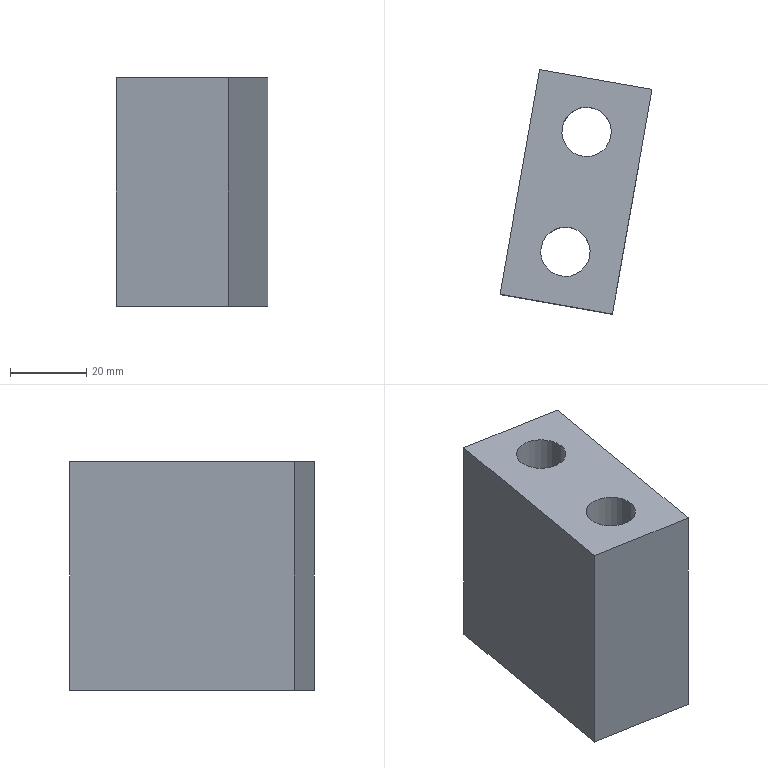Part | NX | features solid 2 | 1 solid | 12 faces | box 39.963 x 64.298 x 60 mm | volume 84815 mm3 | plane 8 | cylinder 4 | commonest cylinder face diameters 13 x2 20 x2
STEP:
#1=CARTESIAN_POINT('',(487.163,-102.147,147.5));
#2=VERTEX_POINT('',#1);
#3=CARTESIAN_POINT('',(493.565,-103.276,147.5));
#4=DIRECTION('',(0.,0.,-1.));
#5=DIRECTION('',(-0.9848,0.1736,0.));
#6=AXIS2_PLACEMENT_3D('',#3,#4,#5);
#7=CIRCLE('',#6,6.5);
#8=EDGE_CURVE('',#2,#2,#7,.F.);
#9=ORIENTED_EDGE('',*,*,#8,.F.);
#10=EDGE_LOOP('',(#9));
#11=FACE_BOUND('',#10,.T.);
#12=CARTESIAN_POINT('',(492.72,-70.633,147.5));
#13=VERTEX_POINT('',#12);
#14=CARTESIAN_POINT('',(499.121,-71.762,147.5));
#15=DIRECTION('',(0.,0.,-1.));
#16=DIRECTION('',(-0.9848,0.1736,0.));
#17=AXIS2_PLACEMENT_3D('',#14,#15,#16);
#18=CIRCLE('',#17,6.5);
#19=EDGE_CURVE('',#13,#13,#18,.F.);
#20=ORIENTED_EDGE('',*,*,#19,.F.);
#21=EDGE_LOOP('',(#20));
#22=FACE_BOUND('',#21,.T.);
#23=CARTESIAN_POINT('',(486.78,-55.37,147.5));
#24=VERTEX_POINT('',#23);
#25=CARTESIAN_POINT('',(516.325,-60.579,147.5));
#26=VERTEX_POINT('',#25);
#27=CARTESIAN_POINT('',(481.856,-54.501,147.5));
#28=DIRECTION('',(-0.9848,0.1736,0.));
#29=VECTOR('',#28,1000.);
#30=LINE('',#27,#29);
#31=EDGE_CURVE('',#24,#26,#30,.F.);
#32=ORIENTED_EDGE('',*,*,#31,.F.);
#33=CARTESIAN_POINT('',(476.362,-114.458,147.5));
#34=VERTEX_POINT('',#33);
#35=CARTESIAN_POINT('',(476.362,-114.458,147.5));
#36=DIRECTION('',(-0.1736,-0.9848,0.));
#37=VECTOR('',#36,1000.);
#38=LINE('',#35,#37);
#39=EDGE_CURVE('',#34,#24,#38,.F.);
#40=ORIENTED_EDGE('',*,*,#39,.F.);
#41=CARTESIAN_POINT('',(505.906,-119.668,147.5));
#42=VERTEX_POINT('',#41);
#43=CARTESIAN_POINT('',(471.438,-113.59,147.5));
#44=DIRECTION('',(-0.9848,0.1736,0.));
#45=VECTOR('',#44,1000.);
#46=LINE('',#43,#45);
#47=EDGE_CURVE('',#34,#42,#46,.F.);
#48=ORIENTED_EDGE('',*,*,#47,.T.);
#49=CARTESIAN_POINT('',(505.906,-119.668,147.5));
#50=DIRECTION('',(-0.1736,-0.9848,0.));
#51=VECTOR('',#50,1000.);
#52=LINE('',#49,#51);
#53=EDGE_CURVE('',#42,#26,#52,.F.);
#54=ORIENTED_EDGE('',*,*,#53,.T.);
#55=EDGE_LOOP('',(#32,#40,#48,#54));
#56=FACE_BOUND('',#55,.T.);
#57=CARTESIAN_POINT('',(471.438,-113.59,147.5));
#58=DIRECTION('',(0.,0.,1.));
#59=DIRECTION('',(0.1736,0.9848,0.));
#60=AXIS2_PLACEMENT_3D('',#57,#58,#59);
#61=PLANE('',#60);
#62=ADVANCED_FACE('',(#11,#22,#56),#61,.T.);
#63=ORIENTED_EDGE('',*,*,#47,.F.);
#64=CARTESIAN_POINT('',(476.362,-114.458,87.5));
#65=VERTEX_POINT('',#64);
#66=CARTESIAN_POINT('',(476.362,-114.458,147.5));
#67=DIRECTION('',(0.,0.,-1.));
#68=VECTOR('',#67,1000.);
#69=LINE('',#66,#68);
#70=EDGE_CURVE('',#34,#65,#69,.T.);
#71=ORIENTED_EDGE('',*,*,#70,.T.);
#72=CARTESIAN_POINT('',(505.906,-119.668,87.5));
#73=VERTEX_POINT('',#72);
#74=CARTESIAN_POINT('',(471.438,-113.59,87.5));
#75=DIRECTION('',(0.9848,-0.1736,0.));
#76=VECTOR('',#75,1000.);
#77=LINE('',#74,#76);
#78=EDGE_CURVE('',#65,#73,#77,.T.);
#79=ORIENTED_EDGE('',*,*,#78,.T.);
#80=CARTESIAN_POINT('',(505.906,-119.668,147.5));
#81=DIRECTION('',(0.,0.,-1.));
#82=VECTOR('',#81,1000.);
#83=LINE('',#80,#82);
#84=EDGE_CURVE('',#42,#73,#83,.T.);
#85=ORIENTED_EDGE('',*,*,#84,.F.);
#86=EDGE_LOOP('',(#63,#71,#79,#85));
#87=FACE_BOUND('',#86,.T.);
#88=CARTESIAN_POINT('',(471.438,-113.59,147.5));
#89=DIRECTION('',(0.1736,0.9848,0.));
#90=DIRECTION('',(0.,0.,-1.));
#91=AXIS2_PLACEMENT_3D('',#88,#89,#90);
#92=PLANE('',#91);
#93=ADVANCED_FACE('',(#87),#92,.F.);
#94=CARTESIAN_POINT('',(483.717,-101.539,87.5));
#95=VERTEX_POINT('',#94);
#96=CARTESIAN_POINT('',(493.565,-103.276,87.5));
#97=DIRECTION('',(0.,0.,-1.));
#98=DIRECTION('',(-0.9848,0.1736,0.));
#99=AXIS2_PLACEMENT_3D('',#96,#97,#98);
#100=CIRCLE('',#99,10.);
#101=EDGE_CURVE('',#95,#95,#100,.T.);
#102=ORIENTED_EDGE('',*,*,#101,.F.);
#103=EDGE_LOOP('',(#102));
#104=FACE_BOUND('',#103,.T.);
#105=CARTESIAN_POINT('',(489.273,-70.025,87.5));
#106=VERTEX_POINT('',#105);
#107=CARTESIAN_POINT('',(499.121,-71.762,87.5));
#108=DIRECTION('',(0.,0.,-1.));
#109=DIRECTION('',(-0.9848,0.1736,0.));
#110=AXIS2_PLACEMENT_3D('',#107,#108,#109);
#111=CIRCLE('',#110,10.);
#112=EDGE_CURVE('',#106,#106,#111,.T.);
#113=ORIENTED_EDGE('',*,*,#112,.F.);
#114=EDGE_LOOP('',(#113));
#115=FACE_BOUND('',#114,.T.);
#116=ORIENTED_EDGE('',*,*,#78,.F.);
#117=CARTESIAN_POINT('',(486.78,-55.37,87.5));
#118=VERTEX_POINT('',#117);
#119=CARTESIAN_POINT('',(476.362,-114.458,87.5));
#120=DIRECTION('',(0.1736,0.9848,0.));
#121=VECTOR('',#120,1000.);
#122=LINE('',#119,#121);
#123=EDGE_CURVE('',#65,#118,#122,.T.);
#124=ORIENTED_EDGE('',*,*,#123,.T.);
#125=CARTESIAN_POINT('',(516.325,-60.579,87.5));
#126=VERTEX_POINT('',#125);
#127=CARTESIAN_POINT('',(481.856,-54.501,87.5));
#128=DIRECTION('',(-0.9848,0.1736,0.));
#129=VECTOR('',#128,1000.);
#130=LINE('',#127,#129);
#131=EDGE_CURVE('',#118,#126,#130,.F.);
#132=ORIENTED_EDGE('',*,*,#131,.T.);
#133=CARTESIAN_POINT('',(505.906,-119.668,87.5));
#134=DIRECTION('',(0.1736,0.9848,0.));
#135=VECTOR('',#134,1000.);
#136=LINE('',#133,#135);
#137=EDGE_CURVE('',#73,#126,#136,.T.);
#138=ORIENTED_EDGE('',*,*,#137,.F.);
#139=EDGE_LOOP('',(#116,#124,#132,#138));
#140=FACE_BOUND('',#139,.T.);
#141=CARTESIAN_POINT('',(471.438,-113.59,87.5));
#142=DIRECTION('',(0.,0.,1.));
#143=DIRECTION('',(0.1736,0.9848,0.));
#144=AXIS2_PLACEMENT_3D('',#141,#142,#143);
#145=PLANE('',#144);
#146=ADVANCED_FACE('',(#104,#115,#140),#145,.F.);
#147=CARTESIAN_POINT('',(486.78,-55.37,147.5));
#148=DIRECTION('',(0.,0.,1.));
#149=VECTOR('',#148,1000.);
#150=LINE('',#147,#149);
#151=EDGE_CURVE('',#24,#118,#150,.F.);
#152=ORIENTED_EDGE('',*,*,#151,.F.);
#153=ORIENTED_EDGE('',*,*,#31,.T.);
#154=CARTESIAN_POINT('',(516.325,-60.579,147.5));
#155=DIRECTION('',(0.,0.,1.));
#156=VECTOR('',#155,1000.);
#157=LINE('',#154,#156);
#158=EDGE_CURVE('',#26,#126,#157,.F.);
#159=ORIENTED_EDGE('',*,*,#158,.T.);
#160=ORIENTED_EDGE('',*,*,#131,.F.);
#161=EDGE_LOOP('',(#152,#153,#159,#160));
#162=FACE_BOUND('',#161,.T.);
#163=CARTESIAN_POINT('',(481.856,-54.501,147.5));
#164=DIRECTION('',(0.1736,0.9848,0.));
#165=DIRECTION('',(0.,0.,-1.));
#166=AXIS2_PLACEMENT_3D('',#163,#164,#165);
#167=PLANE('',#166);
#168=ADVANCED_FACE('',(#162),#167,.T.);
#169=ORIENTED_EDGE('',*,*,#137,.T.);
#170=ORIENTED_EDGE('',*,*,#158,.F.);
#171=ORIENTED_EDGE('',*,*,#53,.F.);
#172=ORIENTED_EDGE('',*,*,#84,.T.);
#173=EDGE_LOOP('',(#169,#170,#171,#172));
#174=FACE_BOUND('',#173,.T.);
#175=CARTESIAN_POINT('',(505.906,-119.668,147.5));
#176=DIRECTION('',(0.9848,-0.1736,0.));
#177=DIRECTION('',(0.,0.,1.));
#178=AXIS2_PLACEMENT_3D('',#175,#176,#177);
#179=PLANE('',#178);
#180=ADVANCED_FACE('',(#174),#179,.T.);
#181=ORIENTED_EDGE('',*,*,#123,.F.);
#182=ORIENTED_EDGE('',*,*,#70,.F.);
#183=ORIENTED_EDGE('',*,*,#39,.T.);
#184=ORIENTED_EDGE('',*,*,#151,.T.);
#185=EDGE_LOOP('',(#181,#182,#183,#184));
#186=FACE_BOUND('',#185,.T.);
#187=CARTESIAN_POINT('',(476.362,-114.458,147.5));
#188=DIRECTION('',(0.9848,-0.1736,0.));
#189=DIRECTION('',(0.,0.,1.));
#190=AXIS2_PLACEMENT_3D('',#187,#188,#189);
#191=PLANE('',#190);
#192=ADVANCED_FACE('',(#186),#191,.F.);
#193=CARTESIAN_POINT('',(492.72,-70.633,107.5));
#194=VERTEX_POINT('',#193);
#195=CARTESIAN_POINT('',(499.121,-71.762,107.5));
#196=DIRECTION('',(0.,0.,-1.));
#197=DIRECTION('',(-0.9848,0.1736,0.));
#198=AXIS2_PLACEMENT_3D('',#195,#196,#197);
#199=CIRCLE('',#198,6.5);
#200=EDGE_CURVE('',#194,#194,#199,.T.);
#201=ORIENTED_EDGE('',*,*,#200,.T.);
#202=EDGE_LOOP('',(#201));
#203=FACE_BOUND('',#202,.T.);
#204=ORIENTED_EDGE('',*,*,#19,.T.);
#205=EDGE_LOOP('',(#204));
#206=FACE_BOUND('',#205,.T.);
#207=CARTESIAN_POINT('',(499.121,-71.762,167.5));
#208=DIRECTION('',(0.,0.,1.));
#209=DIRECTION('',(-0.9848,0.1736,0.));
#210=AXIS2_PLACEMENT_3D('',#207,#208,#209);
#211=CYLINDRICAL_SURFACE('',#210,6.5);
#212=ADVANCED_FACE('',(#203,#206),#211,.F.);
#213=ORIENTED_EDGE('',*,*,#200,.F.);
#214=EDGE_LOOP('',(#213));
#215=FACE_BOUND('',#214,.T.);
#216=CARTESIAN_POINT('',(489.273,-70.025,107.5));
#217=VERTEX_POINT('',#216);
#218=CARTESIAN_POINT('',(499.121,-71.762,107.5));
#219=DIRECTION('',(0.,0.,-1.));
#220=DIRECTION('',(-0.9848,0.1736,0.));
#221=AXIS2_PLACEMENT_3D('',#218,#219,#220);
#222=CIRCLE('',#221,10.);
#223=EDGE_CURVE('',#217,#217,#222,.T.);
#224=ORIENTED_EDGE('',*,*,#223,.T.);
#225=EDGE_LOOP('',(#224));
#226=FACE_BOUND('',#225,.T.);
#227=CARTESIAN_POINT('',(499.469,-69.792,107.5));
#228=DIRECTION('',(0.,0.,1.));
#229=DIRECTION('',(-0.9848,0.1736,0.));
#230=AXIS2_PLACEMENT_3D('',#227,#228,#229);
#231=PLANE('',#230);
#232=ADVANCED_FACE('',(#215,#226),#231,.F.);
#233=ORIENTED_EDGE('',*,*,#223,.F.);
#234=EDGE_LOOP('',(#233));
#235=FACE_BOUND('',#234,.T.);
#236=ORIENTED_EDGE('',*,*,#112,.T.);
#237=EDGE_LOOP('',(#236));
#238=FACE_BOUND('',#237,.T.);
#239=CARTESIAN_POINT('',(499.121,-71.762,87.5));
#240=DIRECTION('',(0.,0.,1.));
#241=DIRECTION('',(-0.9848,0.1736,0.));
#242=AXIS2_PLACEMENT_3D('',#239,#240,#241);
#243=CYLINDRICAL_SURFACE('',#242,10.);
#244=ADVANCED_FACE('',(#235,#238),#243,.F.);
#245=CARTESIAN_POINT('',(487.163,-102.147,107.5));
#246=VERTEX_POINT('',#245);
#247=CARTESIAN_POINT('',(493.565,-103.276,107.5));
#248=DIRECTION('',(0.,0.,-1.));
#249=DIRECTION('',(-0.9848,0.1736,0.));
#250=AXIS2_PLACEMENT_3D('',#247,#248,#249);
#251=CIRCLE('',#250,6.5);
#252=EDGE_CURVE('',#246,#246,#251,.T.);
#253=ORIENTED_EDGE('',*,*,#252,.T.);
#254=EDGE_LOOP('',(#253));
#255=FACE_BOUND('',#254,.T.);
#256=ORIENTED_EDGE('',*,*,#8,.T.);
#257=EDGE_LOOP('',(#256));
#258=FACE_BOUND('',#257,.T.);
#259=CARTESIAN_POINT('',(493.565,-103.276,167.5));
#260=DIRECTION('',(0.,0.,1.));
#261=DIRECTION('',(-0.9848,0.1736,0.));
#262=AXIS2_PLACEMENT_3D('',#259,#260,#261);
#263=CYLINDRICAL_SURFACE('',#262,6.5);
#264=ADVANCED_FACE('',(#255,#258),#263,.F.);
#265=ORIENTED_EDGE('',*,*,#252,.F.);
#266=EDGE_LOOP('',(#265));
#267=FACE_BOUND('',#266,.T.);
#268=CARTESIAN_POINT('',(483.717,-101.539,107.5));
#269=VERTEX_POINT('',#268);
#270=CARTESIAN_POINT('',(493.565,-103.276,107.5));
#271=DIRECTION('',(0.,0.,-1.));
#272=DIRECTION('',(-0.9848,0.1736,0.));
#273=AXIS2_PLACEMENT_3D('',#270,#271,#272);
#274=CIRCLE('',#273,10.);
#275=EDGE_CURVE('',#269,#269,#274,.T.);
#276=ORIENTED_EDGE('',*,*,#275,.T.);
#277=EDGE_LOOP('',(#276));
#278=FACE_BOUND('',#277,.T.);
#279=CARTESIAN_POINT('',(493.217,-105.245,107.5));
#280=DIRECTION('',(0.,0.,1.));
#281=DIRECTION('',(-0.9848,0.1736,0.));
#282=AXIS2_PLACEMENT_3D('',#279,#280,#281);
#283=PLANE('',#282);
#284=ADVANCED_FACE('',(#267,#278),#283,.F.);
#285=ORIENTED_EDGE('',*,*,#275,.F.);
#286=EDGE_LOOP('',(#285));
#287=FACE_BOUND('',#286,.T.);
#288=ORIENTED_EDGE('',*,*,#101,.T.);
#289=EDGE_LOOP('',(#288));
#290=FACE_BOUND('',#289,.T.);
#291=CARTESIAN_POINT('',(493.565,-103.276,87.5));
#292=DIRECTION('',(0.,0.,1.));
#293=DIRECTION('',(-0.9848,0.1736,0.));
#294=AXIS2_PLACEMENT_3D('',#291,#292,#293);
#295=CYLINDRICAL_SURFACE('',#294,10.);
#296=ADVANCED_FACE('',(#287,#290),#295,.F.);
#297=CLOSED_SHELL('',(#62,#93,#146,#168,#180,#192,#212,#232,#244,#264,#284,#296));
#298=MANIFOLD_SOLID_BREP('',#297);
#299=(LENGTH_UNIT()NAMED_UNIT(*)SI_UNIT(.MILLI.,.METRE.));
#300=UNCERTAINTY_MEASURE_WITH_UNIT(LENGTH_MEASURE(0.00001),#299,'','');
#301=(NAMED_UNIT(*)PLANE_ANGLE_UNIT()SI_UNIT($,.RADIAN.));
#302=(NAMED_UNIT(*)SI_UNIT($,.STERADIAN.)SOLID_ANGLE_UNIT());
#303=(GEOMETRIC_REPRESENTATION_CONTEXT(3)GLOBAL_UNCERTAINTY_ASSIGNED_CONTEXT((#300))GLOBAL_UNIT_ASSIGNED_CONTEXT((#299,#301,#302))REPRESENTATION_CONTEXT('',''));
#304=ADVANCED_BREP_SHAPE_REPRESENTATION('',(#298),#303);